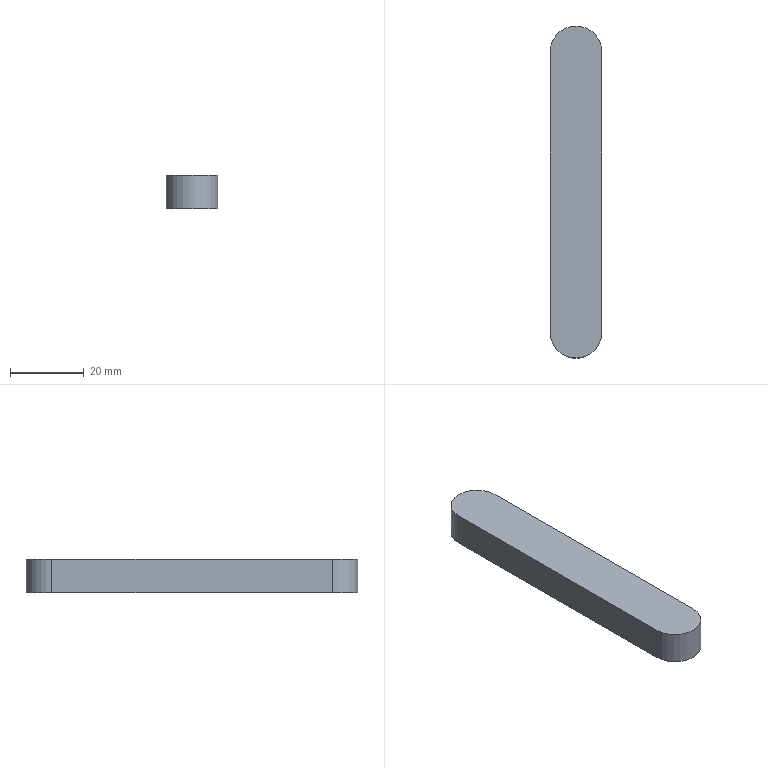Part | STEP file | PN_0059_default | 1 solid | 7 faces | box 14 x 90 x 9 mm | volume 10961 mm3 | plane 4 | cylinder 3 | commonest cylinder face diameters 14 x3
STEP:
#1=CARTESIAN_POINT('',(0.,0.,0.));
#2=DIRECTION('',(0.,0.,1.));
#3=DIRECTION('',(1.,0.,0.));
#4=AXIS2_PLACEMENT_3D('',#1,#2,#3);
#5=CARTESIAN_POINT('',(0.,45.,4.5));
#6=VERTEX_POINT('',#5);
#7=CARTESIAN_POINT('',(-7.,38.,4.5));
#8=VERTEX_POINT('',#7);
#9=CARTESIAN_POINT('',(0.,38.,4.5));
#10=DIRECTION('',(0.,0.,1.));
#11=DIRECTION('',(0.,1.,0.));
#12=AXIS2_PLACEMENT_3D('',#9,#10,#11);
#13=CIRCLE('',#12,7.);
#14=CARTESIAN_POINT('',(0.,38.,4.5));
#15=DIRECTION('',(0.,0.,-1.));
#16=DIRECTION('',(0.,1.,0.));
#17=AXIS2_PLACEMENT_3D('',#14,#15,#16);
#18=CYLINDRICAL_SURFACE('',#17,7.);
#19=CARTESIAN_POINT('',(6.283,0.));
#20=DIRECTION('',(-1.,0.));
#21=VECTOR('',#20,1.);
#22=LINE('',#19,#21);
#23=(GEOMETRIC_REPRESENTATION_CONTEXT(2)PARAMETRIC_REPRESENTATION_CONTEXT()REPRESENTATION_CONTEXT('',''));
#24=DEFINITIONAL_REPRESENTATION('',(#22),#23);
#25=PCURVE('',#18,#24);
#26=CARTESIAN_POINT('',(0.,0.,4.5));
#27=DIRECTION('',(0.,0.,1.));
#28=DIRECTION('',(1.,0.,0.));
#29=AXIS2_PLACEMENT_3D('',#26,#27,#28);
#30=PLANE('',#29);
#31=CARTESIAN_POINT('',(0.,38.));
#32=DIRECTION('',(0.,1.));
#33=AXIS2_PLACEMENT_2D('',#31,#32);
#34=CIRCLE('',#33,7.);
#35=(GEOMETRIC_REPRESENTATION_CONTEXT(2)PARAMETRIC_REPRESENTATION_CONTEXT()REPRESENTATION_CONTEXT('',''));
#36=DEFINITIONAL_REPRESENTATION('',(#34),#35);
#37=PCURVE('',#30,#36);
#38=SURFACE_CURVE('',#13,(#25,#37),.PCURVE_S1.);
#39=EDGE_CURVE('',#6,#8,#38,.T.);
#40=ORIENTED_EDGE('',*,*,#39,.F.);
#41=CARTESIAN_POINT('',(0.,45.,-4.5));
#42=VERTEX_POINT('',#41);
#43=CARTESIAN_POINT('',(0.,45.,4.5));
#44=DIRECTION('',(0.,0.,-1.));
#45=VECTOR('',#44,1.);
#46=LINE('',#43,#45);
#47=CARTESIAN_POINT('',(6.283,0.));
#48=DIRECTION('',(0.,1.));
#49=VECTOR('',#48,1.);
#50=LINE('',#47,#49);
#51=(GEOMETRIC_REPRESENTATION_CONTEXT(2)PARAMETRIC_REPRESENTATION_CONTEXT()REPRESENTATION_CONTEXT('',''));
#52=DEFINITIONAL_REPRESENTATION('',(#50),#51);
#53=PCURVE('',#18,#52);
#54=CARTESIAN_POINT('',(0.,38.,4.5));
#55=DIRECTION('',(0.,0.,-1.));
#56=DIRECTION('',(0.,1.,0.));
#57=AXIS2_PLACEMENT_3D('',#54,#55,#56);
#58=CYLINDRICAL_SURFACE('',#57,7.);
#59=CARTESIAN_POINT('',(0.,0.));
#60=DIRECTION('',(0.,1.));
#61=VECTOR('',#60,1.);
#62=LINE('',#59,#61);
#63=(GEOMETRIC_REPRESENTATION_CONTEXT(2)PARAMETRIC_REPRESENTATION_CONTEXT()REPRESENTATION_CONTEXT('',''));
#64=DEFINITIONAL_REPRESENTATION('',(#62),#63);
#65=PCURVE('',#58,#64);
#66=SURFACE_CURVE('',#46,(#53,#65),.PCURVE_S1.);
#67=EDGE_CURVE('',#6,#42,#66,.T.);
#68=ORIENTED_EDGE('',*,*,#67,.T.);
#69=CARTESIAN_POINT('',(-7.,38.,-4.5));
#70=VERTEX_POINT('',#69);
#71=CARTESIAN_POINT('',(0.,38.,-4.5));
#72=DIRECTION('',(0.,0.,1.));
#73=DIRECTION('',(0.,1.,0.));
#74=AXIS2_PLACEMENT_3D('',#71,#72,#73);
#75=CIRCLE('',#74,7.);
#76=CARTESIAN_POINT('',(6.283,9.));
#77=DIRECTION('',(-1.,0.));
#78=VECTOR('',#77,1.);
#79=LINE('',#76,#78);
#80=(GEOMETRIC_REPRESENTATION_CONTEXT(2)PARAMETRIC_REPRESENTATION_CONTEXT()REPRESENTATION_CONTEXT('',''));
#81=DEFINITIONAL_REPRESENTATION('',(#79),#80);
#82=PCURVE('',#18,#81);
#83=CARTESIAN_POINT('',(0.,0.,-4.5));
#84=DIRECTION('',(0.,0.,1.));
#85=DIRECTION('',(1.,0.,0.));
#86=AXIS2_PLACEMENT_3D('',#83,#84,#85);
#87=PLANE('',#86);
#88=CARTESIAN_POINT('',(0.,38.));
#89=DIRECTION('',(0.,1.));
#90=AXIS2_PLACEMENT_2D('',#88,#89);
#91=CIRCLE('',#90,7.);
#92=(GEOMETRIC_REPRESENTATION_CONTEXT(2)PARAMETRIC_REPRESENTATION_CONTEXT()REPRESENTATION_CONTEXT('',''));
#93=DEFINITIONAL_REPRESENTATION('',(#91),#92);
#94=PCURVE('',#87,#93);
#95=SURFACE_CURVE('',#75,(#82,#94),.PCURVE_S1.);
#96=EDGE_CURVE('',#42,#70,#95,.T.);
#97=ORIENTED_EDGE('',*,*,#96,.T.);
#98=CARTESIAN_POINT('',(-7.,38.,4.5));
#99=DIRECTION('',(0.,0.,-1.));
#100=VECTOR('',#99,1.);
#101=LINE('',#98,#100);
#102=CARTESIAN_POINT('',(4.712,0.));
#103=DIRECTION('',(0.,1.));
#104=VECTOR('',#103,1.);
#105=LINE('',#102,#104);
#106=(GEOMETRIC_REPRESENTATION_CONTEXT(2)PARAMETRIC_REPRESENTATION_CONTEXT()REPRESENTATION_CONTEXT('',''));
#107=DEFINITIONAL_REPRESENTATION('',(#105),#106);
#108=PCURVE('',#18,#107);
#109=CARTESIAN_POINT('',(-7.,38.,4.5));
#110=DIRECTION('',(-1.,0.,0.));
#111=DIRECTION('',(0.,0.,1.));
#112=AXIS2_PLACEMENT_3D('',#109,#110,#111);
#113=PLANE('',#112);
#114=CARTESIAN_POINT('',(0.,0.));
#115=DIRECTION('',(-1.,0.));
#116=VECTOR('',#115,1.);
#117=LINE('',#114,#116);
#118=(GEOMETRIC_REPRESENTATION_CONTEXT(2)PARAMETRIC_REPRESENTATION_CONTEXT()REPRESENTATION_CONTEXT('',''));
#119=DEFINITIONAL_REPRESENTATION('',(#117),#118);
#120=PCURVE('',#113,#119);
#121=SURFACE_CURVE('',#101,(#108,#120),.PCURVE_S1.);
#122=EDGE_CURVE('',#8,#70,#121,.T.);
#123=ORIENTED_EDGE('',*,*,#122,.F.);
#124=EDGE_LOOP('',(#40,#68,#97,#123));
#125=FACE_BOUND('',#124,.T.);
#126=ADVANCED_FACE('',(#125),#18,.T.);
#127=CARTESIAN_POINT('',(-7.,-38.,4.5));
#128=VERTEX_POINT('',#127);
#129=CARTESIAN_POINT('',(7.,-38.,4.5));
#130=VERTEX_POINT('',#129);
#131=CARTESIAN_POINT('',(0.,-38.,4.5));
#132=DIRECTION('',(0.,0.,1.));
#133=DIRECTION('',(0.,1.,0.));
#134=AXIS2_PLACEMENT_3D('',#131,#132,#133);
#135=CIRCLE('',#134,7.);
#136=CARTESIAN_POINT('',(0.,-38.));
#137=DIRECTION('',(0.,1.));
#138=AXIS2_PLACEMENT_2D('',#136,#137);
#139=CIRCLE('',#138,7.);
#140=(GEOMETRIC_REPRESENTATION_CONTEXT(2)PARAMETRIC_REPRESENTATION_CONTEXT()REPRESENTATION_CONTEXT('',''));
#141=DEFINITIONAL_REPRESENTATION('',(#139),#140);
#142=PCURVE('',#30,#141);
#143=CARTESIAN_POINT('',(0.,-38.,4.5));
#144=DIRECTION('',(0.,0.,-1.));
#145=DIRECTION('',(0.,1.,0.));
#146=AXIS2_PLACEMENT_3D('',#143,#144,#145);
#147=CYLINDRICAL_SURFACE('',#146,7.);
#148=CARTESIAN_POINT('',(6.283,0.));
#149=DIRECTION('',(-1.,0.));
#150=VECTOR('',#149,1.);
#151=LINE('',#148,#150);
#152=(GEOMETRIC_REPRESENTATION_CONTEXT(2)PARAMETRIC_REPRESENTATION_CONTEXT()REPRESENTATION_CONTEXT('',''));
#153=DEFINITIONAL_REPRESENTATION('',(#151),#152);
#154=PCURVE('',#147,#153);
#155=SURFACE_CURVE('',#135,(#142,#154),.PCURVE_S1.);
#156=EDGE_CURVE('',#128,#130,#155,.T.);
#157=ORIENTED_EDGE('',*,*,#156,.T.);
#158=CARTESIAN_POINT('',(7.,38.,4.5));
#159=VERTEX_POINT('',#158);
#160=CARTESIAN_POINT('',(7.,-38.,4.5));
#161=DIRECTION('',(0.,1.,0.));
#162=VECTOR('',#161,1.);
#163=LINE('',#160,#162);
#164=CARTESIAN_POINT('',(7.,-38.));
#165=DIRECTION('',(0.,1.));
#166=VECTOR('',#165,1.);
#167=LINE('',#164,#166);
#168=(GEOMETRIC_REPRESENTATION_CONTEXT(2)PARAMETRIC_REPRESENTATION_CONTEXT()REPRESENTATION_CONTEXT('',''));
#169=DEFINITIONAL_REPRESENTATION('',(#167),#168);
#170=PCURVE('',#30,#169);
#171=CARTESIAN_POINT('',(7.,-38.,4.5));
#172=DIRECTION('',(1.,0.,0.));
#173=DIRECTION('',(0.,1.,0.));
#174=AXIS2_PLACEMENT_3D('',#171,#172,#173);
#175=PLANE('',#174);
#176=CARTESIAN_POINT('',(0.,0.));
#177=DIRECTION('',(1.,0.));
#178=VECTOR('',#177,1.);
#179=LINE('',#176,#178);
#180=(GEOMETRIC_REPRESENTATION_CONTEXT(2)PARAMETRIC_REPRESENTATION_CONTEXT()REPRESENTATION_CONTEXT('',''));
#181=DEFINITIONAL_REPRESENTATION('',(#179),#180);
#182=PCURVE('',#175,#181);
#183=SURFACE_CURVE('',#163,(#170,#182),.PCURVE_S1.);
#184=EDGE_CURVE('',#130,#159,#183,.T.);
#185=ORIENTED_EDGE('',*,*,#184,.T.);
#186=CARTESIAN_POINT('',(0.,38.,4.5));
#187=DIRECTION('',(0.,0.,1.));
#188=DIRECTION('',(0.,1.,0.));
#189=AXIS2_PLACEMENT_3D('',#186,#187,#188);
#190=CIRCLE('',#189,7.);
#191=CARTESIAN_POINT('',(0.,38.));
#192=DIRECTION('',(0.,1.));
#193=AXIS2_PLACEMENT_2D('',#191,#192);
#194=CIRCLE('',#193,7.);
#195=(GEOMETRIC_REPRESENTATION_CONTEXT(2)PARAMETRIC_REPRESENTATION_CONTEXT()REPRESENTATION_CONTEXT('',''));
#196=DEFINITIONAL_REPRESENTATION('',(#194),#195);
#197=PCURVE('',#30,#196);
#198=CARTESIAN_POINT('',(6.283,0.));
#199=DIRECTION('',(-1.,0.));
#200=VECTOR('',#199,1.);
#201=LINE('',#198,#200);
#202=(GEOMETRIC_REPRESENTATION_CONTEXT(2)PARAMETRIC_REPRESENTATION_CONTEXT()REPRESENTATION_CONTEXT('',''));
#203=DEFINITIONAL_REPRESENTATION('',(#201),#202);
#204=PCURVE('',#58,#203);
#205=SURFACE_CURVE('',#190,(#197,#204),.PCURVE_S1.);
#206=EDGE_CURVE('',#159,#6,#205,.T.);
#207=ORIENTED_EDGE('',*,*,#206,.T.);
#208=ORIENTED_EDGE('',*,*,#39,.T.);
#209=CARTESIAN_POINT('',(-7.,38.,4.5));
#210=DIRECTION('',(0.,-1.,0.));
#211=VECTOR('',#210,1.);
#212=LINE('',#209,#211);
#213=CARTESIAN_POINT('',(-7.,38.));
#214=DIRECTION('',(0.,-1.));
#215=VECTOR('',#214,1.);
#216=LINE('',#213,#215);
#217=(GEOMETRIC_REPRESENTATION_CONTEXT(2)PARAMETRIC_REPRESENTATION_CONTEXT()REPRESENTATION_CONTEXT('',''));
#218=DEFINITIONAL_REPRESENTATION('',(#216),#217);
#219=PCURVE('',#30,#218);
#220=CARTESIAN_POINT('',(0.,0.));
#221=DIRECTION('',(0.,-1.));
#222=VECTOR('',#221,1.);
#223=LINE('',#220,#222);
#224=(GEOMETRIC_REPRESENTATION_CONTEXT(2)PARAMETRIC_REPRESENTATION_CONTEXT()REPRESENTATION_CONTEXT('',''));
#225=DEFINITIONAL_REPRESENTATION('',(#223),#224);
#226=PCURVE('',#113,#225);
#227=SURFACE_CURVE('',#212,(#219,#226),.PCURVE_S1.);
#228=EDGE_CURVE('',#8,#128,#227,.T.);
#229=ORIENTED_EDGE('',*,*,#228,.T.);
#230=EDGE_LOOP('',(#157,#185,#207,#208,#229));
#231=FACE_BOUND('',#230,.T.);
#232=ADVANCED_FACE('',(#231),#30,.T.);
#233=CARTESIAN_POINT('',(7.,-38.,-4.5));
#234=VERTEX_POINT('',#233);
#235=CARTESIAN_POINT('',(7.,38.,-4.5));
#236=VERTEX_POINT('',#235);
#237=CARTESIAN_POINT('',(7.,-38.,-4.5));
#238=DIRECTION('',(0.,1.,0.));
#239=VECTOR('',#238,1.);
#240=LINE('',#237,#239);
#241=CARTESIAN_POINT('',(7.,-38.));
#242=DIRECTION('',(0.,1.));
#243=VECTOR('',#242,1.);
#244=LINE('',#241,#243);
#245=(GEOMETRIC_REPRESENTATION_CONTEXT(2)PARAMETRIC_REPRESENTATION_CONTEXT()REPRESENTATION_CONTEXT('',''));
#246=DEFINITIONAL_REPRESENTATION('',(#244),#245);
#247=PCURVE('',#87,#246);
#248=CARTESIAN_POINT('',(0.,-9.));
#249=DIRECTION('',(1.,0.));
#250=VECTOR('',#249,1.);
#251=LINE('',#248,#250);
#252=(GEOMETRIC_REPRESENTATION_CONTEXT(2)PARAMETRIC_REPRESENTATION_CONTEXT()REPRESENTATION_CONTEXT('',''));
#253=DEFINITIONAL_REPRESENTATION('',(#251),#252);
#254=PCURVE('',#175,#253);
#255=SURFACE_CURVE('',#240,(#247,#254),.PCURVE_S1.);
#256=EDGE_CURVE('',#234,#236,#255,.T.);
#257=ORIENTED_EDGE('',*,*,#256,.F.);
#258=CARTESIAN_POINT('',(-7.,-38.,-4.5));
#259=VERTEX_POINT('',#258);
#260=CARTESIAN_POINT('',(0.,-38.,-4.5));
#261=DIRECTION('',(0.,0.,1.));
#262=DIRECTION('',(0.,1.,0.));
#263=AXIS2_PLACEMENT_3D('',#260,#261,#262);
#264=CIRCLE('',#263,7.);
#265=CARTESIAN_POINT('',(0.,-38.));
#266=DIRECTION('',(0.,1.));
#267=AXIS2_PLACEMENT_2D('',#265,#266);
#268=CIRCLE('',#267,7.);
#269=(GEOMETRIC_REPRESENTATION_CONTEXT(2)PARAMETRIC_REPRESENTATION_CONTEXT()REPRESENTATION_CONTEXT('',''));
#270=DEFINITIONAL_REPRESENTATION('',(#268),#269);
#271=PCURVE('',#87,#270);
#272=CARTESIAN_POINT('',(6.283,9.));
#273=DIRECTION('',(-1.,0.));
#274=VECTOR('',#273,1.);
#275=LINE('',#272,#274);
#276=(GEOMETRIC_REPRESENTATION_CONTEXT(2)PARAMETRIC_REPRESENTATION_CONTEXT()REPRESENTATION_CONTEXT('',''));
#277=DEFINITIONAL_REPRESENTATION('',(#275),#276);
#278=PCURVE('',#147,#277);
#279=SURFACE_CURVE('',#264,(#271,#278),.PCURVE_S1.);
#280=EDGE_CURVE('',#259,#234,#279,.T.);
#281=ORIENTED_EDGE('',*,*,#280,.F.);
#282=CARTESIAN_POINT('',(-7.,38.,-4.5));
#283=DIRECTION('',(0.,-1.,0.));
#284=VECTOR('',#283,1.);
#285=LINE('',#282,#284);
#286=CARTESIAN_POINT('',(-7.,38.));
#287=DIRECTION('',(0.,-1.));
#288=VECTOR('',#287,1.);
#289=LINE('',#286,#288);
#290=(GEOMETRIC_REPRESENTATION_CONTEXT(2)PARAMETRIC_REPRESENTATION_CONTEXT()REPRESENTATION_CONTEXT('',''));
#291=DEFINITIONAL_REPRESENTATION('',(#289),#290);
#292=PCURVE('',#87,#291);
#293=CARTESIAN_POINT('',(-9.,0.));
#294=DIRECTION('',(0.,-1.));
#295=VECTOR('',#294,1.);
#296=LINE('',#293,#295);
#297=(GEOMETRIC_REPRESENTATION_CONTEXT(2)PARAMETRIC_REPRESENTATION_CONTEXT()REPRESENTATION_CONTEXT('',''));
#298=DEFINITIONAL_REPRESENTATION('',(#296),#297);
#299=PCURVE('',#113,#298);
#300=SURFACE_CURVE('',#285,(#292,#299),.PCURVE_S1.);
#301=EDGE_CURVE('',#70,#259,#300,.T.);
#302=ORIENTED_EDGE('',*,*,#301,.F.);
#303=ORIENTED_EDGE('',*,*,#96,.F.);
#304=CARTESIAN_POINT('',(0.,38.,-4.5));
#305=DIRECTION('',(0.,0.,1.));
#306=DIRECTION('',(0.,1.,0.));
#307=AXIS2_PLACEMENT_3D('',#304,#305,#306);
#308=CIRCLE('',#307,7.);
#309=CARTESIAN_POINT('',(0.,38.));
#310=DIRECTION('',(0.,1.));
#311=AXIS2_PLACEMENT_2D('',#309,#310);
#312=CIRCLE('',#311,7.);
#313=(GEOMETRIC_REPRESENTATION_CONTEXT(2)PARAMETRIC_REPRESENTATION_CONTEXT()REPRESENTATION_CONTEXT('',''));
#314=DEFINITIONAL_REPRESENTATION('',(#312),#313);
#315=PCURVE('',#87,#314);
#316=CARTESIAN_POINT('',(6.283,9.));
#317=DIRECTION('',(-1.,0.));
#318=VECTOR('',#317,1.);
#319=LINE('',#316,#318);
#320=(GEOMETRIC_REPRESENTATION_CONTEXT(2)PARAMETRIC_REPRESENTATION_CONTEXT()REPRESENTATION_CONTEXT('',''));
#321=DEFINITIONAL_REPRESENTATION('',(#319),#320);
#322=PCURVE('',#58,#321);
#323=SURFACE_CURVE('',#308,(#315,#322),.PCURVE_S1.);
#324=EDGE_CURVE('',#236,#42,#323,.T.);
#325=ORIENTED_EDGE('',*,*,#324,.F.);
#326=EDGE_LOOP('',(#257,#281,#302,#303,#325));
#327=FACE_BOUND('',#326,.T.);
#328=ADVANCED_FACE('',(#327),#87,.F.);
#329=ORIENTED_EDGE('',*,*,#280,.T.);
#330=CARTESIAN_POINT('',(7.,-38.,4.5));
#331=DIRECTION('',(0.,0.,-1.));
#332=VECTOR('',#331,1.);
#333=LINE('',#330,#332);
#334=CARTESIAN_POINT('',(1.571,0.));
#335=DIRECTION('',(0.,1.));
#336=VECTOR('',#335,1.);
#337=LINE('',#334,#336);
#338=(GEOMETRIC_REPRESENTATION_CONTEXT(2)PARAMETRIC_REPRESENTATION_CONTEXT()REPRESENTATION_CONTEXT('',''));
#339=DEFINITIONAL_REPRESENTATION('',(#337),#338);
#340=PCURVE('',#147,#339);
#341=CARTESIAN_POINT('',(0.,0.));
#342=DIRECTION('',(0.,-1.));
#343=VECTOR('',#342,1.);
#344=LINE('',#341,#343);
#345=(GEOMETRIC_REPRESENTATION_CONTEXT(2)PARAMETRIC_REPRESENTATION_CONTEXT()REPRESENTATION_CONTEXT('',''));
#346=DEFINITIONAL_REPRESENTATION('',(#344),#345);
#347=PCURVE('',#175,#346);
#348=SURFACE_CURVE('',#333,(#340,#347),.PCURVE_S1.);
#349=EDGE_CURVE('',#130,#234,#348,.T.);
#350=ORIENTED_EDGE('',*,*,#349,.F.);
#351=ORIENTED_EDGE('',*,*,#156,.F.);
#352=CARTESIAN_POINT('',(-7.,-38.,4.5));
#353=DIRECTION('',(0.,0.,-1.));
#354=VECTOR('',#353,1.);
#355=LINE('',#352,#354);
#356=CARTESIAN_POINT('',(4.712,0.));
#357=DIRECTION('',(0.,1.));
#358=VECTOR('',#357,1.);
#359=LINE('',#356,#358);
#360=(GEOMETRIC_REPRESENTATION_CONTEXT(2)PARAMETRIC_REPRESENTATION_CONTEXT()REPRESENTATION_CONTEXT('',''));
#361=DEFINITIONAL_REPRESENTATION('',(#359),#360);
#362=PCURVE('',#147,#361);
#363=CARTESIAN_POINT('',(0.,-76.));
#364=DIRECTION('',(-1.,0.));
#365=VECTOR('',#364,1.);
#366=LINE('',#363,#365);
#367=(GEOMETRIC_REPRESENTATION_CONTEXT(2)PARAMETRIC_REPRESENTATION_CONTEXT()REPRESENTATION_CONTEXT('',''));
#368=DEFINITIONAL_REPRESENTATION('',(#366),#367);
#369=PCURVE('',#113,#368);
#370=SURFACE_CURVE('',#355,(#362,#369),.PCURVE_S1.);
#371=EDGE_CURVE('',#128,#259,#370,.T.);
#372=ORIENTED_EDGE('',*,*,#371,.T.);
#373=EDGE_LOOP('',(#329,#350,#351,#372));
#374=FACE_BOUND('',#373,.T.);
#375=ADVANCED_FACE('',(#374),#147,.T.);
#376=ORIENTED_EDGE('',*,*,#301,.T.);
#377=ORIENTED_EDGE('',*,*,#371,.F.);
#378=ORIENTED_EDGE('',*,*,#228,.F.);
#379=ORIENTED_EDGE('',*,*,#122,.T.);
#380=EDGE_LOOP('',(#376,#377,#378,#379));
#381=FACE_BOUND('',#380,.T.);
#382=ADVANCED_FACE('',(#381),#113,.T.);
#383=ORIENTED_EDGE('',*,*,#67,.F.);
#384=ORIENTED_EDGE('',*,*,#206,.F.);
#385=CARTESIAN_POINT('',(7.,38.,4.5));
#386=DIRECTION('',(0.,0.,-1.));
#387=VECTOR('',#386,1.);
#388=LINE('',#385,#387);
#389=CARTESIAN_POINT('',(1.571,0.));
#390=DIRECTION('',(0.,1.));
#391=VECTOR('',#390,1.);
#392=LINE('',#389,#391);
#393=(GEOMETRIC_REPRESENTATION_CONTEXT(2)PARAMETRIC_REPRESENTATION_CONTEXT()REPRESENTATION_CONTEXT('',''));
#394=DEFINITIONAL_REPRESENTATION('',(#392),#393);
#395=PCURVE('',#58,#394);
#396=CARTESIAN_POINT('',(76.,0.));
#397=DIRECTION('',(0.,-1.));
#398=VECTOR('',#397,1.);
#399=LINE('',#396,#398);
#400=(GEOMETRIC_REPRESENTATION_CONTEXT(2)PARAMETRIC_REPRESENTATION_CONTEXT()REPRESENTATION_CONTEXT('',''));
#401=DEFINITIONAL_REPRESENTATION('',(#399),#400);
#402=PCURVE('',#175,#401);
#403=SURFACE_CURVE('',#388,(#395,#402),.PCURVE_S1.);
#404=EDGE_CURVE('',#159,#236,#403,.T.);
#405=ORIENTED_EDGE('',*,*,#404,.T.);
#406=ORIENTED_EDGE('',*,*,#324,.T.);
#407=EDGE_LOOP('',(#383,#384,#405,#406));
#408=FACE_BOUND('',#407,.T.);
#409=ADVANCED_FACE('',(#408),#58,.T.);
#410=ORIENTED_EDGE('',*,*,#256,.T.);
#411=ORIENTED_EDGE('',*,*,#404,.F.);
#412=ORIENTED_EDGE('',*,*,#184,.F.);
#413=ORIENTED_EDGE('',*,*,#349,.T.);
#414=EDGE_LOOP('',(#410,#411,#412,#413));
#415=FACE_BOUND('',#414,.T.);
#416=ADVANCED_FACE('',(#415),#175,.T.);
#417=CLOSED_SHELL('',(#126,#232,#328,#375,#382,#409,#416));
#418=MANIFOLD_SOLID_BREP('',#417);
#419=(LENGTH_UNIT()NAMED_UNIT(*)SI_UNIT(.MILLI.,.METRE.));
#420=UNCERTAINTY_MEASURE_WITH_UNIT(LENGTH_MEASURE(0.0000001),#419,'','');
#421=(NAMED_UNIT(*)PLANE_ANGLE_UNIT()SI_UNIT($,.RADIAN.));
#422=(NAMED_UNIT(*)SI_UNIT($,.STERADIAN.)SOLID_ANGLE_UNIT());
#423=(GEOMETRIC_REPRESENTATION_CONTEXT(3)GLOBAL_UNCERTAINTY_ASSIGNED_CONTEXT((#420))GLOBAL_UNIT_ASSIGNED_CONTEXT((#419,#421,#422))REPRESENTATION_CONTEXT('',''));
#424=ADVANCED_BREP_SHAPE_REPRESENTATION('',(#4,#418),#423);